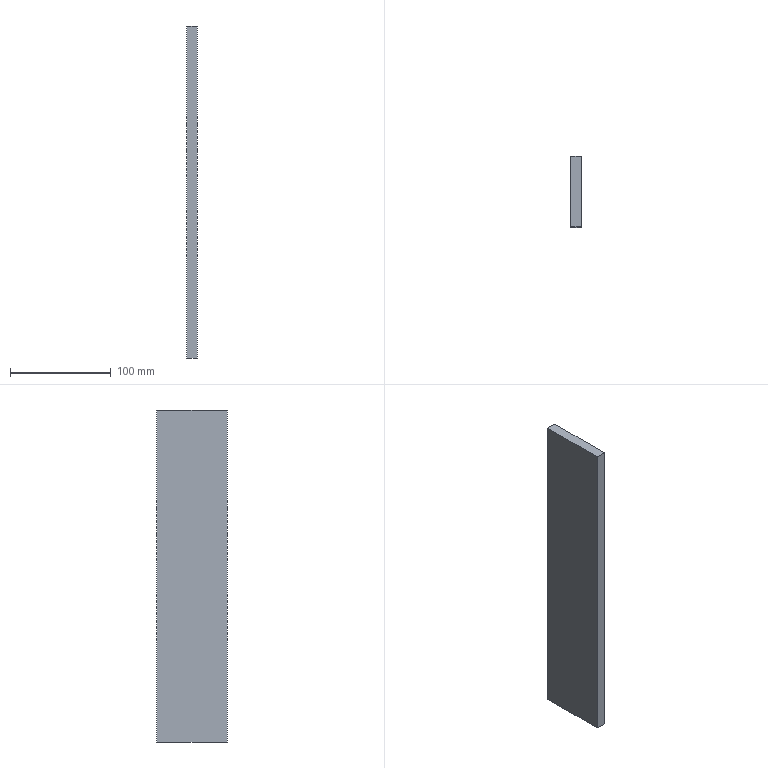Part | SolidWorks | 1 solid | 6 faces | box 10 x 70 x 330 mm | volume 231000 mm3 | plane 6
STEP:
#1=CARTESIAN_POINT('',(5.,0.,165.));
#2=VERTEX_POINT('',#1);
#3=CARTESIAN_POINT('',(5.,0.,-165.));
#4=VERTEX_POINT('',#3);
#5=CARTESIAN_POINT('',(5.,0.,-165.));
#6=DIRECTION('',(0.,0.,-1.));
#7=VECTOR('',#6,1000.);
#8=LINE('',#5,#7);
#9=EDGE_CURVE('',#2,#4,#8,.T.);
#10=ORIENTED_EDGE('',*,*,#9,.T.);
#11=CARTESIAN_POINT('',(5.,70.,-165.));
#12=VERTEX_POINT('',#11);
#13=CARTESIAN_POINT('',(5.,70.,-165.));
#14=DIRECTION('',(0.,-1.,0.));
#15=VECTOR('',#14,1000.);
#16=LINE('',#13,#15);
#17=EDGE_CURVE('',#12,#4,#16,.T.);
#18=ORIENTED_EDGE('',*,*,#17,.F.);
#19=CARTESIAN_POINT('',(5.,70.,165.));
#20=VERTEX_POINT('',#19);
#21=CARTESIAN_POINT('',(5.,70.,-165.));
#22=DIRECTION('',(0.,0.,-1.));
#23=VECTOR('',#22,1000.);
#24=LINE('',#21,#23);
#25=EDGE_CURVE('',#20,#12,#24,.T.);
#26=ORIENTED_EDGE('',*,*,#25,.F.);
#27=CARTESIAN_POINT('',(5.,70.,165.));
#28=DIRECTION('',(0.,-1.,0.));
#29=VECTOR('',#28,1000.);
#30=LINE('',#27,#29);
#31=EDGE_CURVE('',#20,#2,#30,.T.);
#32=ORIENTED_EDGE('',*,*,#31,.T.);
#33=EDGE_LOOP('',(#10,#18,#26,#32));
#34=FACE_OUTER_BOUND('',#33,.T.);
#35=CARTESIAN_POINT('',(5.,70.,-165.));
#36=DIRECTION('',(-1.,0.,0.));
#37=DIRECTION('',(0.,0.,1.));
#38=AXIS2_PLACEMENT_3D('',#35,#36,#37);
#39=PLANE('',#38);
#40=ADVANCED_FACE('',(#34),#39,.F.);
#41=CARTESIAN_POINT('',(-5.,0.,-165.));
#42=VERTEX_POINT('',#41);
#43=CARTESIAN_POINT('',(-5.,0.,-165.));
#44=DIRECTION('',(-1.,0.,0.));
#45=VECTOR('',#44,1000.);
#46=LINE('',#43,#45);
#47=EDGE_CURVE('',#4,#42,#46,.T.);
#48=ORIENTED_EDGE('',*,*,#47,.T.);
#49=CARTESIAN_POINT('',(-5.,70.,-165.));
#50=VERTEX_POINT('',#49);
#51=CARTESIAN_POINT('',(-5.,70.,-165.));
#52=DIRECTION('',(0.,-1.,0.));
#53=VECTOR('',#52,1000.);
#54=LINE('',#51,#53);
#55=EDGE_CURVE('',#50,#42,#54,.T.);
#56=ORIENTED_EDGE('',*,*,#55,.F.);
#57=CARTESIAN_POINT('',(-5.,70.,-165.));
#58=DIRECTION('',(-1.,0.,0.));
#59=VECTOR('',#58,1000.);
#60=LINE('',#57,#59);
#61=EDGE_CURVE('',#12,#50,#60,.T.);
#62=ORIENTED_EDGE('',*,*,#61,.F.);
#63=ORIENTED_EDGE('',*,*,#17,.T.);
#64=EDGE_LOOP('',(#48,#56,#62,#63));
#65=FACE_OUTER_BOUND('',#64,.T.);
#66=CARTESIAN_POINT('',(-5.,70.,-165.));
#67=DIRECTION('',(0.,0.,1.));
#68=DIRECTION('',(1.,0.,0.));
#69=AXIS2_PLACEMENT_3D('',#66,#67,#68);
#70=PLANE('',#69);
#71=ADVANCED_FACE('',(#65),#70,.F.);
#72=CARTESIAN_POINT('',(-5.,0.,165.));
#73=VERTEX_POINT('',#72);
#74=CARTESIAN_POINT('',(-5.,0.,-165.));
#75=DIRECTION('',(0.,0.,1.));
#76=VECTOR('',#75,1000.);
#77=LINE('',#74,#76);
#78=EDGE_CURVE('',#42,#73,#77,.T.);
#79=ORIENTED_EDGE('',*,*,#78,.T.);
#80=CARTESIAN_POINT('',(-5.,70.,165.));
#81=VERTEX_POINT('',#80);
#82=CARTESIAN_POINT('',(-5.,70.,165.));
#83=DIRECTION('',(0.,-1.,0.));
#84=VECTOR('',#83,1000.);
#85=LINE('',#82,#84);
#86=EDGE_CURVE('',#81,#73,#85,.T.);
#87=ORIENTED_EDGE('',*,*,#86,.F.);
#88=CARTESIAN_POINT('',(-5.,70.,-165.));
#89=DIRECTION('',(0.,0.,1.));
#90=VECTOR('',#89,1000.);
#91=LINE('',#88,#90);
#92=EDGE_CURVE('',#50,#81,#91,.T.);
#93=ORIENTED_EDGE('',*,*,#92,.F.);
#94=ORIENTED_EDGE('',*,*,#55,.T.);
#95=EDGE_LOOP('',(#79,#87,#93,#94));
#96=FACE_OUTER_BOUND('',#95,.T.);
#97=CARTESIAN_POINT('',(-5.,70.,-165.));
#98=DIRECTION('',(1.,0.,0.));
#99=DIRECTION('',(0.,0.,-1.));
#100=AXIS2_PLACEMENT_3D('',#97,#98,#99);
#101=PLANE('',#100);
#102=ADVANCED_FACE('',(#96),#101,.F.);
#103=CARTESIAN_POINT('',(-5.,0.,165.));
#104=DIRECTION('',(1.,0.,0.));
#105=VECTOR('',#104,1000.);
#106=LINE('',#103,#105);
#107=EDGE_CURVE('',#73,#2,#106,.T.);
#108=ORIENTED_EDGE('',*,*,#107,.T.);
#109=ORIENTED_EDGE('',*,*,#31,.F.);
#110=CARTESIAN_POINT('',(-5.,70.,165.));
#111=DIRECTION('',(1.,0.,0.));
#112=VECTOR('',#111,1000.);
#113=LINE('',#110,#112);
#114=EDGE_CURVE('',#81,#20,#113,.T.);
#115=ORIENTED_EDGE('',*,*,#114,.F.);
#116=ORIENTED_EDGE('',*,*,#86,.T.);
#117=EDGE_LOOP('',(#108,#109,#115,#116));
#118=FACE_OUTER_BOUND('',#117,.T.);
#119=CARTESIAN_POINT('',(-5.,70.,165.));
#120=DIRECTION('',(0.,0.,-1.));
#121=DIRECTION('',(-1.,0.,0.));
#122=AXIS2_PLACEMENT_3D('',#119,#120,#121);
#123=PLANE('',#122);
#124=ADVANCED_FACE('',(#118),#123,.F.);
#125=ORIENTED_EDGE('',*,*,#25,.T.);
#126=ORIENTED_EDGE('',*,*,#61,.T.);
#127=ORIENTED_EDGE('',*,*,#92,.T.);
#128=ORIENTED_EDGE('',*,*,#114,.T.);
#129=EDGE_LOOP('',(#125,#126,#127,#128));
#130=FACE_OUTER_BOUND('',#129,.T.);
#131=CARTESIAN_POINT('',(0.,70.,0.));
#132=DIRECTION('',(0.,1.,0.));
#133=DIRECTION('',(0.,0.,1.));
#134=AXIS2_PLACEMENT_3D('',#131,#132,#133);
#135=PLANE('',#134);
#136=ADVANCED_FACE('',(#130),#135,.T.);
#137=ORIENTED_EDGE('',*,*,#9,.F.);
#138=ORIENTED_EDGE('',*,*,#107,.F.);
#139=ORIENTED_EDGE('',*,*,#78,.F.);
#140=ORIENTED_EDGE('',*,*,#47,.F.);
#141=EDGE_LOOP('',(#137,#138,#139,#140));
#142=FACE_OUTER_BOUND('',#141,.T.);
#143=CARTESIAN_POINT('',(0.,0.,0.));
#144=DIRECTION('',(0.,1.,0.));
#145=DIRECTION('',(0.,0.,1.));
#146=AXIS2_PLACEMENT_3D('',#143,#144,#145);
#147=PLANE('',#146);
#148=ADVANCED_FACE('',(#142),#147,.F.);
#149=CLOSED_SHELL('',(#40,#71,#102,#124,#136,#148));
#150=MANIFOLD_SOLID_BREP('',#149);
#151=CARTESIAN_POINT('',(0.,0.,0.));
#152=DIRECTION('',(0.,0.,1.));
#153=DIRECTION('',(1.,0.,0.));
#154=AXIS2_PLACEMENT_3D('',#151,#152,#153);
#155=(LENGTH_UNIT()NAMED_UNIT(*)SI_UNIT(.MILLI.,.METRE.));
#156=UNCERTAINTY_MEASURE_WITH_UNIT(LENGTH_MEASURE(0.00001),#155,'','');
#157=(NAMED_UNIT(*)PLANE_ANGLE_UNIT()SI_UNIT($,.RADIAN.));
#158=(NAMED_UNIT(*)SI_UNIT($,.STERADIAN.)SOLID_ANGLE_UNIT());
#159=(GEOMETRIC_REPRESENTATION_CONTEXT(3)GLOBAL_UNCERTAINTY_ASSIGNED_CONTEXT((#156))GLOBAL_UNIT_ASSIGNED_CONTEXT((#155,#157,#158))REPRESENTATION_CONTEXT('',''));
#160=ADVANCED_BREP_SHAPE_REPRESENTATION('',(#150,#154),#159);